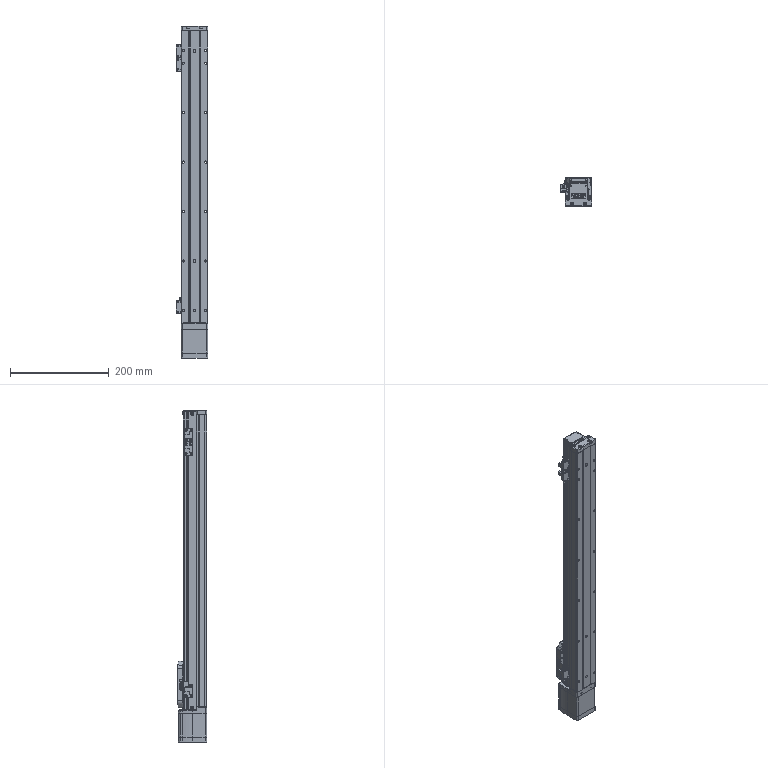Part | SolidWorks | 16 solids | 1825 faces | box 64 x 60 x 671 mm | volume 1247970 mm3 | plane 895 | cylinder 636 | spline 179 | cone 115 | commonest cylinder face diameters 1 x91 2.5 x52 2 x43 3.3 x32 5.5 x32 4.4 x28